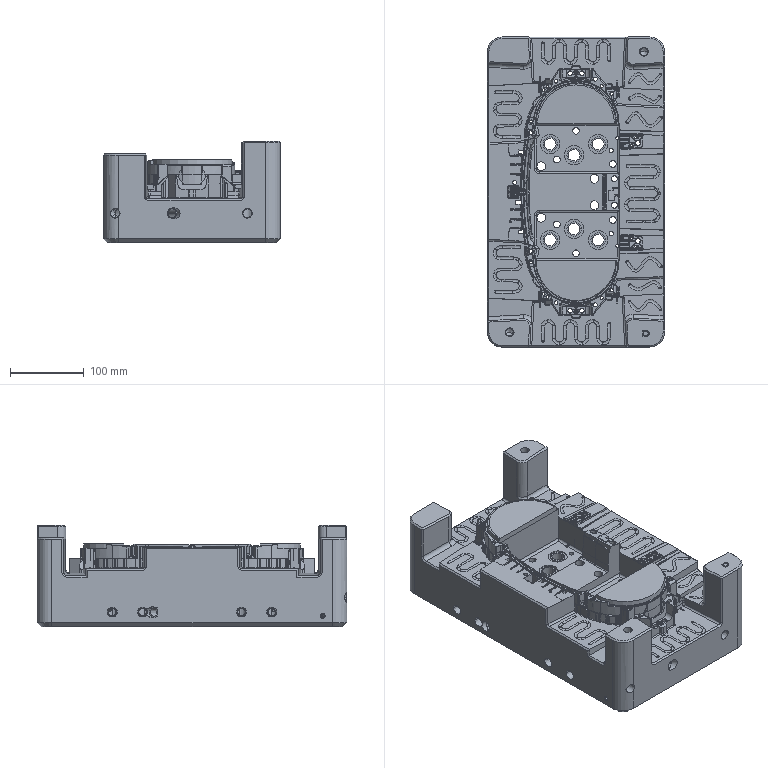Part | Creo | 3 solids | 4164 faces | volume 7732621 mm3 | cylinder 1505 | plane 998 | spline 983 | other 281 | sphere 159 | cone 157 | torus 81 | commonest cylinder face diameters 0.402 x433 1.005 x170 0.804 x78 2.01 x72 10 x62 3 x48